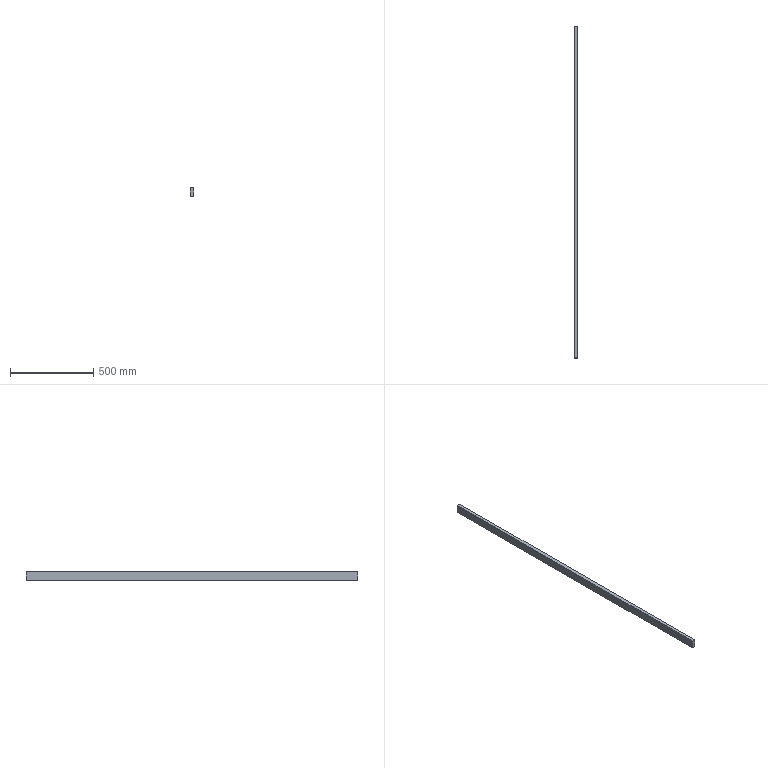Part | SolidWorks | features Extrusion 1 | 1 solid | 6 faces | box 20 x 1996 x 50 mm | volume 1996000 mm3 | plane 6
STEP:
#1=CARTESIAN_POINT('',(0.,1996.,0.));
#2=VERTEX_POINT('',#1);
#3=CARTESIAN_POINT('',(0.,0.,0.));
#4=VERTEX_POINT('',#3);
#5=CARTESIAN_POINT('',(0.,0.,0.));
#6=DIRECTION('',(0.,-1.,0.));
#7=VECTOR('',#6,1000.);
#8=LINE('',#5,#7);
#9=EDGE_CURVE('',#2,#4,#8,.T.);
#10=ORIENTED_EDGE('',*,*,#9,.T.);
#11=CARTESIAN_POINT('',(20.,0.,0.));
#12=VERTEX_POINT('',#11);
#13=CARTESIAN_POINT('',(20.,0.,0.));
#14=DIRECTION('',(-1.,0.,0.));
#15=VECTOR('',#14,1000.);
#16=LINE('',#13,#15);
#17=EDGE_CURVE('',#12,#4,#16,.T.);
#18=ORIENTED_EDGE('',*,*,#17,.F.);
#19=CARTESIAN_POINT('',(20.,1996.,0.));
#20=VERTEX_POINT('',#19);
#21=CARTESIAN_POINT('',(20.,0.,0.));
#22=DIRECTION('',(0.,-1.,0.));
#23=VECTOR('',#22,1000.);
#24=LINE('',#21,#23);
#25=EDGE_CURVE('',#20,#12,#24,.T.);
#26=ORIENTED_EDGE('',*,*,#25,.F.);
#27=CARTESIAN_POINT('',(20.,1996.,0.));
#28=DIRECTION('',(-1.,0.,0.));
#29=VECTOR('',#28,1000.);
#30=LINE('',#27,#29);
#31=EDGE_CURVE('',#20,#2,#30,.T.);
#32=ORIENTED_EDGE('',*,*,#31,.T.);
#33=EDGE_LOOP('',(#10,#18,#26,#32));
#34=FACE_OUTER_BOUND('',#33,.T.);
#35=CARTESIAN_POINT('',(20.,0.,0.));
#36=DIRECTION('',(0.,0.,-1.));
#37=DIRECTION('',(-1.,0.,0.));
#38=AXIS2_PLACEMENT_3D('',#35,#36,#37);
#39=PLANE('',#38);
#40=ADVANCED_FACE('',(#34),#39,.F.);
#41=CARTESIAN_POINT('',(0.,0.,-50.));
#42=VERTEX_POINT('',#41);
#43=CARTESIAN_POINT('',(0.,0.,0.));
#44=DIRECTION('',(0.,0.,-1.));
#45=VECTOR('',#44,1000.);
#46=LINE('',#43,#45);
#47=EDGE_CURVE('',#4,#42,#46,.T.);
#48=ORIENTED_EDGE('',*,*,#47,.T.);
#49=CARTESIAN_POINT('',(20.,0.,-50.));
#50=VERTEX_POINT('',#49);
#51=CARTESIAN_POINT('',(20.,0.,-50.));
#52=DIRECTION('',(-1.,0.,0.));
#53=VECTOR('',#52,1000.);
#54=LINE('',#51,#53);
#55=EDGE_CURVE('',#50,#42,#54,.T.);
#56=ORIENTED_EDGE('',*,*,#55,.F.);
#57=CARTESIAN_POINT('',(20.,0.,0.));
#58=DIRECTION('',(0.,0.,-1.));
#59=VECTOR('',#58,1000.);
#60=LINE('',#57,#59);
#61=EDGE_CURVE('',#12,#50,#60,.T.);
#62=ORIENTED_EDGE('',*,*,#61,.F.);
#63=ORIENTED_EDGE('',*,*,#17,.T.);
#64=EDGE_LOOP('',(#48,#56,#62,#63));
#65=FACE_OUTER_BOUND('',#64,.T.);
#66=CARTESIAN_POINT('',(20.,0.,0.));
#67=DIRECTION('',(0.,1.,0.));
#68=DIRECTION('',(0.,0.,1.));
#69=AXIS2_PLACEMENT_3D('',#66,#67,#68);
#70=PLANE('',#69);
#71=ADVANCED_FACE('',(#65),#70,.F.);
#72=CARTESIAN_POINT('',(0.,1996.,-50.));
#73=VERTEX_POINT('',#72);
#74=CARTESIAN_POINT('',(0.,0.,-50.));
#75=DIRECTION('',(0.,1.,0.));
#76=VECTOR('',#75,1000.);
#77=LINE('',#74,#76);
#78=EDGE_CURVE('',#42,#73,#77,.T.);
#79=ORIENTED_EDGE('',*,*,#78,.T.);
#80=CARTESIAN_POINT('',(20.,1996.,-50.));
#81=VERTEX_POINT('',#80);
#82=CARTESIAN_POINT('',(20.,1996.,-50.));
#83=DIRECTION('',(-1.,0.,0.));
#84=VECTOR('',#83,1000.);
#85=LINE('',#82,#84);
#86=EDGE_CURVE('',#81,#73,#85,.T.);
#87=ORIENTED_EDGE('',*,*,#86,.F.);
#88=CARTESIAN_POINT('',(20.,0.,-50.));
#89=DIRECTION('',(0.,1.,0.));
#90=VECTOR('',#89,1000.);
#91=LINE('',#88,#90);
#92=EDGE_CURVE('',#50,#81,#91,.T.);
#93=ORIENTED_EDGE('',*,*,#92,.F.);
#94=ORIENTED_EDGE('',*,*,#55,.T.);
#95=EDGE_LOOP('',(#79,#87,#93,#94));
#96=FACE_OUTER_BOUND('',#95,.T.);
#97=CARTESIAN_POINT('',(20.,0.,-50.));
#98=DIRECTION('',(0.,0.,1.));
#99=DIRECTION('',(1.,0.,0.));
#100=AXIS2_PLACEMENT_3D('',#97,#98,#99);
#101=PLANE('',#100);
#102=ADVANCED_FACE('',(#96),#101,.F.);
#103=CARTESIAN_POINT('',(0.,1996.,0.));
#104=DIRECTION('',(0.,0.,1.));
#105=VECTOR('',#104,1000.);
#106=LINE('',#103,#105);
#107=EDGE_CURVE('',#73,#2,#106,.T.);
#108=ORIENTED_EDGE('',*,*,#107,.T.);
#109=ORIENTED_EDGE('',*,*,#31,.F.);
#110=CARTESIAN_POINT('',(20.,1996.,0.));
#111=DIRECTION('',(0.,0.,1.));
#112=VECTOR('',#111,1000.);
#113=LINE('',#110,#112);
#114=EDGE_CURVE('',#81,#20,#113,.T.);
#115=ORIENTED_EDGE('',*,*,#114,.F.);
#116=ORIENTED_EDGE('',*,*,#86,.T.);
#117=EDGE_LOOP('',(#108,#109,#115,#116));
#118=FACE_OUTER_BOUND('',#117,.T.);
#119=CARTESIAN_POINT('',(20.,1996.,0.));
#120=DIRECTION('',(0.,-1.,0.));
#121=DIRECTION('',(0.,0.,-1.));
#122=AXIS2_PLACEMENT_3D('',#119,#120,#121);
#123=PLANE('',#122);
#124=ADVANCED_FACE('',(#118),#123,.F.);
#125=ORIENTED_EDGE('',*,*,#25,.T.);
#126=ORIENTED_EDGE('',*,*,#61,.T.);
#127=ORIENTED_EDGE('',*,*,#92,.T.);
#128=ORIENTED_EDGE('',*,*,#114,.T.);
#129=EDGE_LOOP('',(#125,#126,#127,#128));
#130=FACE_OUTER_BOUND('',#129,.T.);
#131=CARTESIAN_POINT('',(20.,0.,0.));
#132=DIRECTION('',(-1.,0.,0.));
#133=DIRECTION('',(0.,0.,1.));
#134=AXIS2_PLACEMENT_3D('',#131,#132,#133);
#135=PLANE('',#134);
#136=ADVANCED_FACE('',(#130),#135,.F.);
#137=ORIENTED_EDGE('',*,*,#9,.F.);
#138=ORIENTED_EDGE('',*,*,#107,.F.);
#139=ORIENTED_EDGE('',*,*,#78,.F.);
#140=ORIENTED_EDGE('',*,*,#47,.F.);
#141=EDGE_LOOP('',(#137,#138,#139,#140));
#142=FACE_OUTER_BOUND('',#141,.T.);
#143=CARTESIAN_POINT('',(0.,0.,0.));
#144=DIRECTION('',(-1.,0.,0.));
#145=DIRECTION('',(0.,0.,1.));
#146=AXIS2_PLACEMENT_3D('',#143,#144,#145);
#147=PLANE('',#146);
#148=ADVANCED_FACE('',(#142),#147,.T.);
#149=CLOSED_SHELL('',(#40,#71,#102,#124,#136,#148));
#150=MANIFOLD_SOLID_BREP('',#149);
#151=CARTESIAN_POINT('',(0.,0.,0.));
#152=DIRECTION('',(0.,0.,1.));
#153=DIRECTION('',(1.,0.,0.));
#154=AXIS2_PLACEMENT_3D('',#151,#152,#153);
#155=(LENGTH_UNIT()NAMED_UNIT(*)SI_UNIT(.MILLI.,.METRE.));
#156=UNCERTAINTY_MEASURE_WITH_UNIT(LENGTH_MEASURE(0.00001),#155,'','');
#157=(NAMED_UNIT(*)PLANE_ANGLE_UNIT()SI_UNIT($,.RADIAN.));
#158=(NAMED_UNIT(*)SI_UNIT($,.STERADIAN.)SOLID_ANGLE_UNIT());
#159=(GEOMETRIC_REPRESENTATION_CONTEXT(3)GLOBAL_UNCERTAINTY_ASSIGNED_CONTEXT((#156))GLOBAL_UNIT_ASSIGNED_CONTEXT((#155,#157,#158))REPRESENTATION_CONTEXT('',''));
#160=ADVANCED_BREP_SHAPE_REPRESENTATION('',(#150,#154),#159);